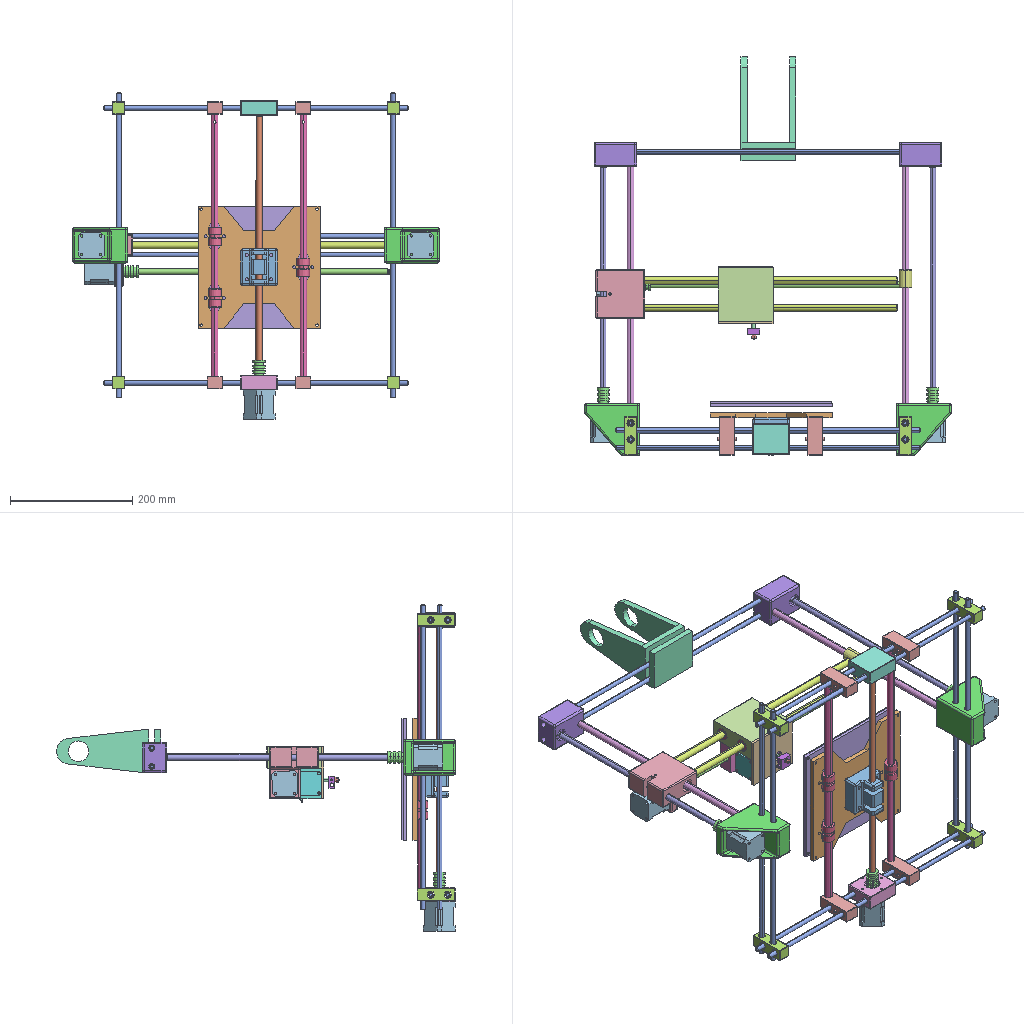Assembly | SolidWorks | 39 different items | 77 placed | box 600 x 653 x 535 mm
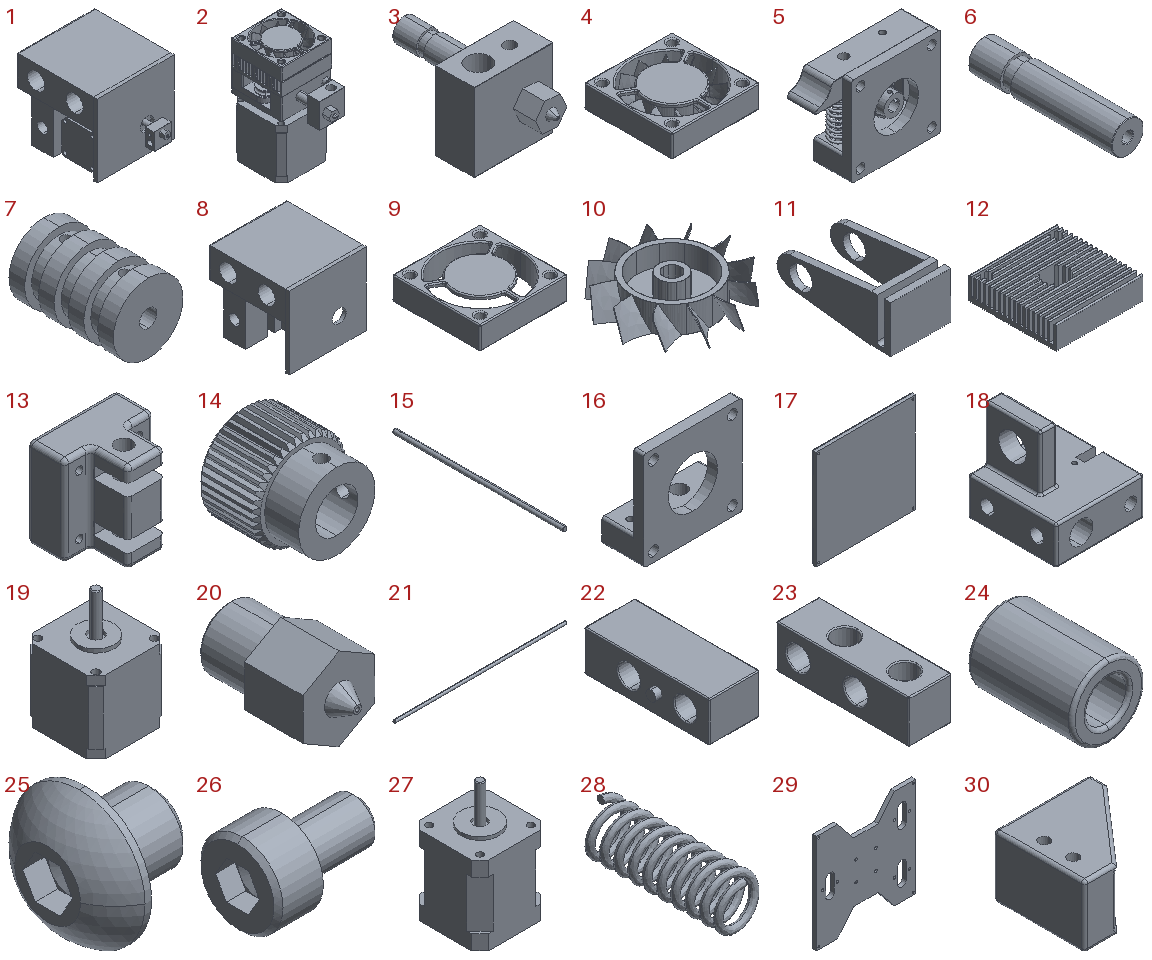Parts list (item | name | quantity | parent item | size | volume | features):
1 | (subassembly) | x1 | - | 90 x 119.5 x 91.979 mm | 440210 mm3 | features InContextFeatHolder 2
2 | (subassembly) | x1 | in 1 | 52.269 x 72.401 x 83.639 mm | 115279 mm3 | -
3 | (subassembly) | x1 | in 2 | 20 x 39.5 x 20 mm | 4094 mm3 | -
4 | (subassembly) | x1 | in 2 | 40 x 40 x 10.5 mm | 24242 mm3 | -
5 | (subassembly) | x1 | in 2 | 52.047 x 17 x 40.013 mm | 16596 mm3 | -
6 | - | x1 | in 3 | 6 x 27 x 6 mm | 611.558 mm3 | features Revolution 1
7 | - | x4 | - | 20 x 30 x 20 mm | 6534 mm3 | features ICE 1, Revolution 1
8 | - | x1 | in 1 | 90 x 94 x 85 mm | 324931 mm3 | features ICE 4, Cut 1, Extrusion 1, Fillet 1
9 | - | x1 | in 4 | 40 x 40 x 10.5 mm | 3410 mm3 | features ICE 3, Fillet 2, Extrusion 1, Shell 1
10 | - | x1 | in 4 | 36.047 x 36.047 x 8.091 mm | 20832 mm3 | features BlendRefSurface 1, CirPattern 1, RefCurve 1, Revolution 1, Thicken 1
11 | - | x1 | - | 90 x 171 x 70 mm | 261901 mm3 | features ICE 2, Extrusion 1, MirrorPattern 1
12 | - | x1 | in 2 | 40 x 40 x 10.5 mm | 8547 mm3 | features ICE 2, Extrusion 1, Fillet 1, LPattern 1, MirrorPattern 1
13 | - | x1 | - | 60 x 50 x 60 mm | 110960 mm3 | features ICE 2, Extrusion 1, Fillet 1
14 | - | x1 | in 5 | 10.985 x 11 x 10.985 mm | 652.018 mm3 | features ICE 3, CirPattern 1, Revolution 1
15 | - | x6 | - | 12 x 450 x 12 mm | 50710 mm3 | features Chamfer 1, Extrusion 1, ICE 1
16 | - | x1 | in 5 | 40 x 17 x 40 mm | 9241 mm3 | features ICE 2, Extrusion 1, Fillet 1
17 | - | x1 | - | 200 x 8 x 200 mm | 318006 mm3 | features ICE 2, Extrusion 1, PLine 1
18 | - | x1 | - | 80 x 80 x 85 mm | 211032 mm3 | features ICE 5, Extrusion 1, Fillet 1
19 | - | x1 | in 2 | 40 x 40 x 64 mm | 61607 mm3 | features ICE 5, Chamfer 2, Extrusion 1, MirrorPattern 1
20 | - | x1 | in 3 | 7 x 12.5 x 8.083 mm | 370.688 mm3 | features ICE 1, Revolution 1
21 | - | x10 | - | 500 x 8 x 8 mm | 25083 mm3 | features Chamfer 1, Extrusion 1
22 | - | x4 | - | 31 x 62 x 20 mm | 24637 mm3 | features ICE 2, Extrusion 1, Fillet 1
23 | - | x4 | - | 20 x 62 x 20 mm | 17160 mm3 | features Extrusion 1, Fillet 1, ICE 1
24 | - | x2 | - | 21 x 30 x 21 mm | 6953 mm3 | features Extrusion 1, Fillet 1
25 | - | x1 | in 5 | 6.2 x 7.6 x 7.6 mm | 113.262 mm3 | features RevCut 2, Cut 1, Fillet 1, LPattern 1, Revolution 1
26 | - | x2 | in 2 | 8 x 5.5 x 5.5 mm | 96.895 mm3 | features CirPattern 3, Cut 3, RevCut 2, Fillet 1, LPattern 1, Revolution 1
27 | - | x4 | - | 42 x 42 x 72 mm | 78719 mm3 | features ICE 5, Chamfer 2, Extrusion 1, MirrorPattern 1
28 | - | x1 | in 5 | 7 x 21 x 7 mm | 148.098 mm3 | features Helix 1, Sweep 1
29 | - | x1 | - | 200 x 8 x 200 mm | 247540 mm3 | features Cut 1, Extrusion 1, ICE 1
30 | - | x2 | - | 90 x 85 x 58 mm | 199222 mm3 | features Fillet 3, ICE 3, Extrusion 1, MirrorPattern 1
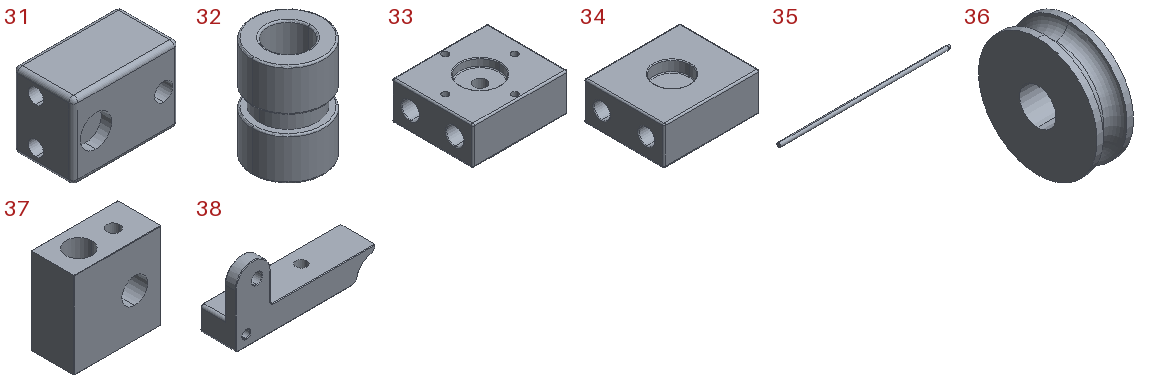31 | - | x2 | - | 70 x 40 x 50 mm | 121422 mm3 | features ICE 3, Extrusion 1, Fillet 1
32 | - | x6 | - | 21 x 21 x 30 mm | 6383 mm3 | features Extrusion 1, Fillet 1, ICE 1
33 | - | x1 | - | 60 x 51 x 24 mm | 57298 mm3 | features ICE 3, Fillet 2, Cut 1, Extrusion 1
34 | - | x1 | - | 60 x 50 x 24 mm | 59794 mm3 | features Fillet 2, ICE 2, Extrusion 1
35 | - | x4 | - | 437 x 10 x 10 mm | 34052 mm3 | features ICE 2, Chamfer 1, Extrusion 1
36 | - | x1 | in 5 | 4 x 13 x 13 mm | 381.449 mm3 | features Revolution 1
37 | - | x1 | in 3 | 20 x 10 x 20 mm | 3112 mm3 | features ICE 3, Extrusion 1, Fillet 1
38 | - | x1 | in 5 | 52 x 13 x 26.5 mm | 6060 mm3 | features Fillet 2, ICE 2, Extrusion 1, HoleWzd 1
39 | right | x1 | - | - | - | -
Mates (type | each side: item.copy, entity, surface, feature):
In the top assembly
Concentric | 22.1 face cylinder Boss-Extrude1 | 23.1 face cylinder Boss-Extrude1 | 2 times
Coincident | 22.1 face plane Boss-Extrude1 | 22.2 face plane Boss-Extrude1 | 2 times
Coincident | 22.2 face plane Boss-Extrude1 | 23.2 face plane Boss-Extrude1 | 2 times
Concentric | 21.1 face cylinder Boss-Extrude1 | 23.1 face cylinder Boss-Extrude1
Concentric | 21.2 face cylinder Boss-Extrude1 | 23.1 face cylinder Boss-Extrude1
Coincident | 21.1 face plane Boss-Extrude1 | 21.2 face plane Boss-Extrude1
Coincident | 23.1 face plane Boss-Extrude1 | 23.3 face plane Boss-Extrude1
Coincident | 23.2 face plane Boss-Extrude1 | 23.4 face plane Boss-Extrude1
DistanceDim | 22.1 face plane Boss-Extrude1 | 23.1 face plane Boss-Extrude1
DistanceDim | 22.1 face plane Boss-Extrude1 | 22.2 face plane Boss-Extrude1
DistanceDim | 23.1 face plane Boss-Extrude1 | 23.2 face plane Boss-Extrude1
DistanceDim | 23.2 face plane Boss-Extrude1 | 23.4 face plane Boss-Extrude1
Width | 21.2 face plane Boss-Extrude1 | 21.2 face plane Boss-Extrude1 | 23.2 face plane Boss-Extrude1 | 23.1 face plane Boss-Extrude1
Concentric | 21.3 face cylinder Boss-Extrude1 | 23.1 face cylinder Cut-Extrude1
Concentric | 21.4 face cylinder Boss-Extrude1 | 23.1 face cylinder Cut-Extrude1
Coincident | 21.4 face plane Boss-Extrude1 | 21.3 face plane Boss-Extrude1
Concentric | 21.5 face cylinder Boss-Extrude1 | 23.2 face cylinder Cut-Extrude1
Concentric | 21.6 face cylinder Boss-Extrude1 | 23.2 face cylinder Cut-Extrude1
Coincident | 21.6 face plane Boss-Extrude1 | 21.5 face plane Boss-Extrude1
Concentric | 21.7 face cylinder Boss-Extrude1 | 23.4 face cylinder Boss-Extrude1
Concentric | 21.8 face cylinder Boss-Extrude1 | 23.4 face cylinder Boss-Extrude1
Coincident | 21.7 face plane Boss-Extrude1 | 21.8 edge
Width | 23.3 face plane Boss-Extrude1 | 23.4 face plane Boss-Extrude1 | 21.7 face plane Boss-Extrude1 | 21.7 face plane Boss-Extrude1
Width | 23.2 face plane Boss-Extrude1 | 23.4 face plane Boss-Extrude1 | 21.5 face plane Boss-Extrude1 | 21.5 face plane Boss-Extrude1
Coincident | 21.4 face plane Boss-Extrude1 | 21.6 edge
Concentric | 21.1 face cylinder Boss-Extrude1 | 34.1 face cylinder Cut-Extrude2
Parallel | 22.1 face plane Boss-Extrude1 | 34.1 face plane Boss-Extrude1
Width | 22.1 face plane Boss-Extrude1 | 22.2 face plane Boss-Extrude1 | 34.1 face plane Boss-Extrude1 | 34.1 face plane Boss-Extrude1
Concentric | 21.7 face cylinder Boss-Extrude1 | 33.1 face cylinder Cut-Extrude2
Concentric | 21.8 face cylinder Boss-Extrude1 | 33.1 face cylinder Cut-Extrude2
Coincident | 33.1 face plane Boss-Extrude1 | 34.1 face plane Boss-Extrude1
Coincident | 29.1 face plane Boss-Extrude1 | 17.1 face plane Boss-Extrude1 | 2 times
DistanceDim | 17.1 face plane Boss-Extrude1 | 29.1 face plane Boss-Extrude1
Coincident | 33.1 face plane Cut-Extrude1 | 7.1 face plane Revolve1
Concentric | 33.1 face cylinder Cut-Extrude1 | 7.1 face cylinder Revolve1
Concentric | 27.1 face cylinder Boss-Extrude4 | 7.2 face cylinder Revolve1
Coincident | 21.9 face plane Boss-Extrude1 | 21.10 face plane Boss-Extrude1
Coincident | 21.8 face plane Boss-Extrude1 | 21.9 face plane Boss-Extrude1
Concentric | 7.3 face cylinder Revolve1 | 27.2 face cylinder Boss-Extrude4
Concentric | 33.1 face cylinder Cut-Extrude3 | 27.3 face cylinder Boss-Extrude4
Coincident | 33.1 face plane Boss-Extrude1 | 27.3 face plane Boss-Extrude2
DistanceDim | 29.1 face plane Boss-Extrude1 | 32.1 face plane Boss-Extrude1
Parallel | 34.1 face plane Boss-Extrude1 | 29.1 face plane Boss-Extrude1
DistanceDim | 32.1 face plane Boss-Extrude1 | 32.2 face plane Boss-Extrude1
Concentric | 21.3 face cylinder Boss-Extrude1 | 23.3 face cylinder Cut-Extrude1
Concentric | 21.7 face cylinder Boss-Extrude1 | 23.3 face cylinder Boss-Extrude1
Concentric | 21.7 face cylinder Boss-Extrude1 | 22.3 face cylinder Boss-Extrude1
Concentric | 21.7 face cylinder Boss-Extrude1 | 22.4 face cylinder Boss-Extrude1
Concentric | 33.1 face cylinder Cut-Extrude5 | 27.3 face cylinder Cut-Extrude2
Coincident | 32.3 face plane Boss-Extrude1 | 32.4 face plane Boss-Extrude1
DistanceDim | 32.4 face plane Boss-Extrude1 | assembly face
DistanceDim | 32.5 face plane Boss-Extrude1 | assembly face
Coincident | 31.1 face plane Boss-Extrude1 | 31.2 face plane Boss-Extrude1
Concentric | 21.10 face cylinder Boss-Extrude1 | 31.2 face cylinder Cut-Extrude1
Concentric | 21.9 face cylinder Boss-Extrude1 | 31.2 face cylinder Cut-Extrude1
Concentric | 21.10 face cylinder Boss-Extrude1 | 31.1 face cylinder Cut-Extrude1
Concentric | 21.9 face cylinder Boss-Extrude1 | 31.1 face cylinder Cut-Extrude1
Concentric | 21.3 face cylinder Boss-Extrude1 | 30.1 face cylinder Cut-Extrude1
Concentric | 21.4 face cylinder Boss-Extrude1 | 30.1 face cylinder Cut-Extrude1
Concentric | 21.5 face cylinder Boss-Extrude1 | 30.2 face cylinder Cut-Extrude1
Concentric | 21.6 face cylinder Boss-Extrude1 | 30.2 face cylinder Cut-Extrude1
Coincident | 24.1 face plane Boss-Extrude1 | 18.1 face plane Boss-Extrude1
Coincident | 27.1 face plane Boss-Extrude2 | 30.1 face plane Boss-Extrude1
Coincident | 7.2 face plane Revolve1 | 30.1 face plane Boss-Extrude1
Coincident | 7.2 face plane Revolve1 | 7.4 face plane Revolve1
Coincident | 27.4 face plane Boss-Extrude2 | 30.2 face plane Boss-Extrude1
Coincident | 8.1 face plane Boss-Extrude1 | 32.4 face plane Boss-Extrude1
Coincident | 8.1 face plane Boss-Extrude1 | 32.5 edge
Width | 23.4 face plane Boss-Extrude1 | 23.2 face plane Boss-Extrude1 | 30.2 face plane Boss-Extrude2 | 30.2 face plane Mirror1
Coincident | 29.1 face plane Boss-Extrude1 | 13.1 face plane Boss-Extrude1
Width | 13.1 face plane Boss-Extrude1 | 13.1 face plane Boss-Extrude1 | 29.1 face plane Boss-Extrude1 | 29.1 face plane Boss-Extrude1
Width | 29.1 face plane Boss-Extrude1 | 29.1 face plane Boss-Extrude1 | 13.1 face plane Boss-Extrude1 | 13.1 face plane Boss-Extrude1
Concentric | 8.1 face cylinder Boss-Extrude1 | 32.5 face cylinder Boss-Extrude1
Concentric | 8.1 face cylinder Boss-Extrude1 | 32.3 face cylinder Boss-Extrude1
Concentric | 8.1 face cylinder Boss-Extrude1 | 32.4 face cylinder Boss-Extrude1
Coincident | 15.1 face plane Boss-Extrude1 | 15.2 face plane Boss-Extrude1
Coincident | 18.1 face plane Cut-Extrude1 | 15.1 face plane Boss-Extrude1
Concentric | 18.1 face cylinder Cut-Extrude1 | 15.1 face cylinder Boss-Extrude1
Concentric | 18.1 face cylinder Cut-Extrude1 | 15.2 face cylinder Boss-Extrude1
Concentric | 8.1 face cylinder Boss-Extrude1 | 15.1 face cylinder Boss-Extrude1
Concentric | 8.1 face cylinder Boss-Extrude1 | 15.2 face cylinder Boss-Extrude1
Coincident | 15.3 face plane Boss-Extrude1 | 15.4 face plane Boss-Extrude1
Coincident | 30.2 face plane Cut-Extrude2 | 15.3 face plane Boss-Extrude1
Concentric | 30.2 face cylinder Cut-Extrude2 | 15.4 face cylinder Boss-Extrude1
Concentric | 30.1 face cylinder Cut-Extrude2 | 15.3 face cylinder Boss-Extrude1
Concentric | 21.9 face cylinder Boss-Extrude1 | 11.1 face cylinder Cut-Extrude1
Parallel | 31.1 face plane Boss-Extrude1 | 11.1 face plane Cut-Extrude1
DistanceDim | 34.1 face plane Cut-Extrude1 | 35.1 face plane Boss-Extrude3
Concentric | 34.1 face cylinder Cut-Extrude1 | 35.1 face cylinder Boss-Extrude1
Concentric | 7.1 face cylinder Revolve1 | 35.1 face cylinder Boss-Extrude1
Concentric | 13.1 face cylinder Boss-Extrude1 | 35.1 face cylinder Boss-Extrude1
Coincident | 35.2 face plane Boss-Extrude1 | 35.3 face plane Boss-Extrude1
DistanceDim | 35.2 face plane Boss-Extrude3 | 31.2 face plane Cut-Extrude3
Concentric | 7.4 face cylinder Revolve1 | 35.3 face cylinder Boss-Extrude1
Concentric | 27.4 face cylinder Boss-Extrude4 | 35.3 face cylinder Boss-Extrude1
Concentric | 7.4 face cylinder Revolve1 | 30.2 face cylinder Cut-Extrude2
Concentric | 31.1 face cylinder Cut-Extrude3 | 35.2 face cylinder Boss-Extrude1
Concentric | 7.2 face cylinder Revolve1 | 35.2 face cylinder Boss-Extrude1
Concentric | 27.1 face cylinder Boss-Extrude4 | 30.1 face cylinder Cut-Extrude2
Coincident | 30.1 face plane Boss-Extrude2 | 30.2 face plane Mirror1
Width | 30.1 face plane Boss-Extrude2 | 30.1 face plane Mirror1 | 23.3 face plane Boss-Extrude1 | 23.1 face plane Boss-Extrude1
Concentric | 27.2 face cylinder Boss-Extrude4 | 35.4 face cylinder Boss-Extrude1
Coincident | 27.2 face plane Boss-Extrude2 | 18.1 face plane Boss-Extrude1
Coincident | 7.3 face plane Revolve1 | 18.1 face plane Boss-Extrude1
Coincident | 15.5 face plane Boss-Extrude1 | 15.6 face plane Boss-Extrude1
Coincident | 22.4 face plane Cut-Extrude1 | 15.5 face plane Boss-Extrude1
Concentric | 22.3 face cylinder Cut-Extrude1 | 15.5 face cylinder Boss-Extrude1
Concentric | 22.4 face cylinder Cut-Extrude1 | 15.6 face cylinder Boss-Extrude1
Concentric | 32.2 face cylinder Boss-Extrude1 | 15.6 face cylinder Boss-Extrude1
Concentric | 32.1 face cylinder Boss-Extrude1 | 15.6 face cylinder Boss-Extrude1
Concentric | 32.6 face cylinder Boss-Extrude1 | 15.5 face cylinder Boss-Extrude1
DistanceDim | 29.1 face plane Boss-Extrude1 | 32.6 face plane Boss-Extrude1
Parallel | 27.1 face plane Boss-Extrude1 | 30.1 face plane Boss-Extrude1
Concentric | 18.1 face cylinder Boss-Extrude1 | 15.4 face cylinder Boss-Extrude1
Concentric | 24.1 face cylinder Boss-Extrude1 | 15.4 face cylinder Boss-Extrude1
Concentric | 24.2 face cylinder Boss-Extrude1 | 15.3 face cylinder Boss-Extrude1
In subassembly 1
Coordinate | 8.2 select_type:25 | 1.1 select_type:11
DistanceDim | 8.2 face plane Boss-Extrude1 | 19.1 face plane Boss-Extrude1
Coincident | 8.2 face plane Boss-Extrude4 | 19.1 face plane Boss-Extrude1
Coincident | 8.2 face plane Boss-Extrude2 | 19.1 face plane Boss-Extrude2
In subassembly 2
Concentric | 16.1 face cylinder Cut-Extrude1 | 19.2 face cylinder Cut-Extrude2 | 2 times
DistanceDim | 16.1 face plane Boss-Extrude1 | 19.2 face plane Boss-Extrude2
Coincident | 38.1 face plane Boss-Extrude1 | 12.1 face plane Boss-Extrude1
Coincident | 12.1 edge | 9.1 face plane Boss-Extrude2
Coincident | 12.1 face plane Boss-Extrude1 | 9.1 face plane Boss-Extrude1 | 2 times
Concentric | 16.1 face cylinder Cut-Extrude1 | 9.1 face cylinder Cut-Extrude1
Concentric | 16.1 face cylinder Cut-Extrude2 | 6.1 face cylinder Revolve1
DistanceDim | 16.1 face plane Boss-Extrude1 | 37.1 face plane Boss-Extrude1
Parallel | 9.1 face plane Boss-Extrude1 | 37.1 face plane Boss-Extrude1
Concentric | 38.1 face cylinder Cut-Extrude2 | 26.1 face cylinder Base-Revolve
Coincident | 38.1 face plane Boss-Extrude1 | 26.1 face plane Base-Revolve
Concentric | 16.1 face cylinder Cut-Extrude2 | 26.2 face cylinder Base-Revolve
Coincident | 16.1 face plane Boss-Extrude1 | 26.2 face plane Base-Revolve
Concentric | 19.2 face cylinder Cut-Extrude2 | 9.1 face cylinder Cut-Extrude1
In subassembly 3
Concentric | 37.2 face cylinder Boss-Extrude1 | 20.1 face cylinder Revolve1
Coincident | 37.2 face plane Boss-Extrude1 | 20.1 face plane Boss-Extrude1
Coincident | 6.2 face plane Revolve1 | 20.1 face plane Revolve1
Concentric | 37.2 face cylinder Boss-Extrude1 | 6.2 face cylinder Revolve1
In subassembly 5
Concentric | 16.2 face cylinder Cut-Extrude1 | 38.2 face cylinder CBORE for M2.5 Pan Head Machine Screw1
Concentric | 38.2 face cylinder Boss-Extrude2 | 36.1 face cylinder Revolve1
Coincident | 38.2 face plane Boss-Extrude2 | 36.1 face plane Revolve1
Coincident | 16.2 face plane Boss-Extrude1 | 38.2 face plane Boss-Extrude1
Coincident | 38.2 axis | 28.1 plane
Parallel | 16.2 face plane Boss-Extrude1 | 28.1 plane | 2 times
Concentric | 36.1 face cylinder Revolve1 | 25.1 face cylinder BaseBody
Coincident | 36.1 face plane Revolve1 | 25.1 face plane BaseBody
Concentric | 16.2 face cylinder Cut-Extrude1 | 14.1 face cylinder Revolve1
Coincident | 36.1 face plane Revolve1 | 14.1 face plane Revolve1
In subassembly 4
Concentric | 9.2 face cylinder Boss-Extrude3 | 10.1 face cylinder CirPattern1
Coincident | 9.2 face plane Boss-Extrude1 | 10.1 face plane CirPattern1